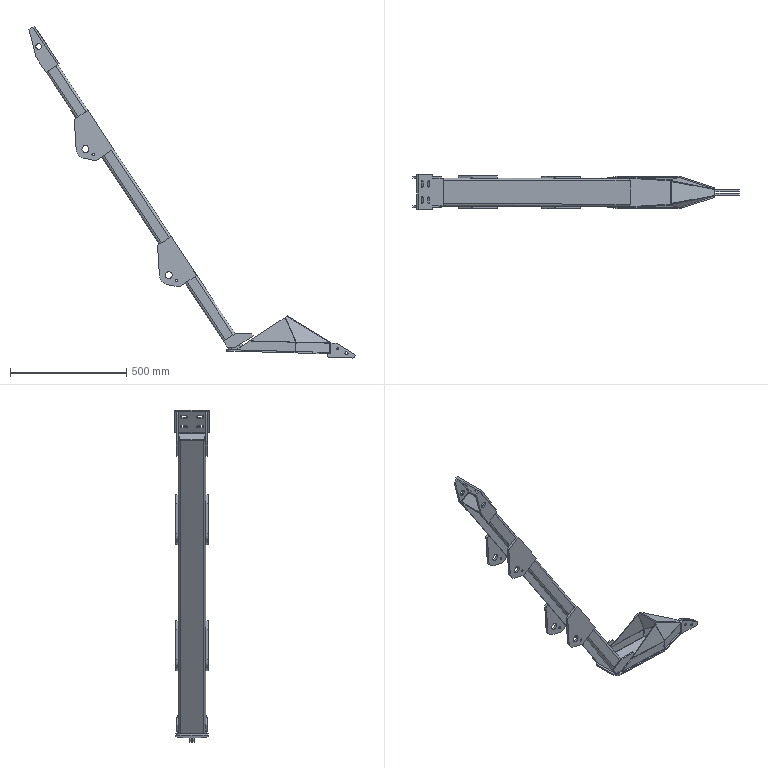Part | STEP file | COMPOUND | 22 solids | 232 faces | box 1402 x 148 x 1427 mm | volume 4524661 mm3 | plane 166 | cylinder 66 | commonest cylinder face diameters 4 x18 13 x10 10 x8 20 x8 30 x4 60 x4